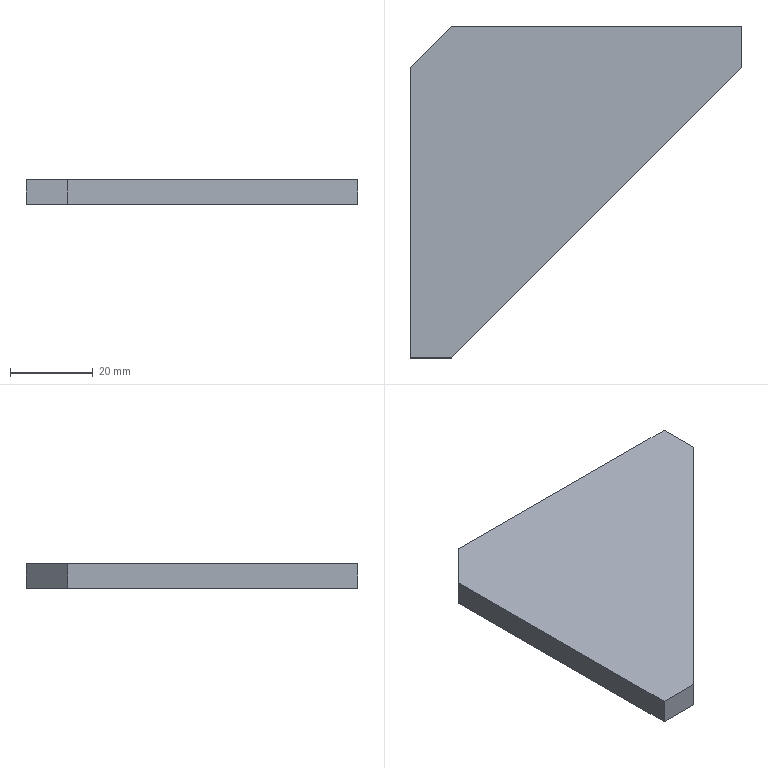Part | SolidWorks | features BaseBody 1 | 1 solid | 8 faces | box 80 x 80 x 6 mm | volume 23400 mm3 | plane 8
STEP:
#1=CARTESIAN_POINT('',(80.,-10.,0.));
#2=VERTEX_POINT('',#1);
#3=CARTESIAN_POINT('',(80.,0.,0.));
#4=VERTEX_POINT('',#3);
#5=CARTESIAN_POINT('',(80.,0.,0.));
#6=DIRECTION('',(0.,1.,0.));
#7=VECTOR('',#6,1000.);
#8=LINE('',#5,#7);
#9=EDGE_CURVE('',#2,#4,#8,.T.);
#10=ORIENTED_EDGE('',*,*,#9,.T.);
#11=CARTESIAN_POINT('',(10.,0.,0.));
#12=VERTEX_POINT('',#11);
#13=CARTESIAN_POINT('',(10.,0.,0.));
#14=DIRECTION('',(-1.,0.,0.));
#15=VECTOR('',#14,1000.);
#16=LINE('',#13,#15);
#17=EDGE_CURVE('',#4,#12,#16,.T.);
#18=ORIENTED_EDGE('',*,*,#17,.T.);
#19=CARTESIAN_POINT('',(0.,-10.,0.));
#20=VERTEX_POINT('',#19);
#21=CARTESIAN_POINT('',(0.,-10.,0.));
#22=DIRECTION('',(-0.7071,-0.7071,0.));
#23=VECTOR('',#22,1000.);
#24=LINE('',#21,#23);
#25=EDGE_CURVE('',#12,#20,#24,.T.);
#26=ORIENTED_EDGE('',*,*,#25,.T.);
#27=CARTESIAN_POINT('',(0.,-80.,0.));
#28=VERTEX_POINT('',#27);
#29=CARTESIAN_POINT('',(0.,-80.,0.));
#30=DIRECTION('',(0.,-1.,0.));
#31=VECTOR('',#30,1000.);
#32=LINE('',#29,#31);
#33=EDGE_CURVE('',#20,#28,#32,.T.);
#34=ORIENTED_EDGE('',*,*,#33,.T.);
#35=CARTESIAN_POINT('',(10.,-80.,0.));
#36=VERTEX_POINT('',#35);
#37=CARTESIAN_POINT('',(10.,-80.,0.));
#38=DIRECTION('',(1.,0.,0.));
#39=VECTOR('',#38,1000.);
#40=LINE('',#37,#39);
#41=EDGE_CURVE('',#28,#36,#40,.T.);
#42=ORIENTED_EDGE('',*,*,#41,.T.);
#43=CARTESIAN_POINT('',(80.,-10.,0.));
#44=DIRECTION('',(0.7071,0.7071,0.));
#45=VECTOR('',#44,1000.);
#46=LINE('',#43,#45);
#47=EDGE_CURVE('',#36,#2,#46,.T.);
#48=ORIENTED_EDGE('',*,*,#47,.T.);
#49=EDGE_LOOP('',(#10,#18,#26,#34,#42,#48));
#50=FACE_OUTER_BOUND('',#49,.T.);
#51=CARTESIAN_POINT('',(0.,0.,0.));
#52=DIRECTION('',(0.,0.,-1.));
#53=DIRECTION('',(0.,-1.,0.));
#54=AXIS2_PLACEMENT_3D('',#51,#52,#53);
#55=PLANE('',#54);
#56=ADVANCED_FACE('',(#50),#55,.F.);
#57=CARTESIAN_POINT('',(80.,-10.,-6.));
#58=VERTEX_POINT('',#57);
#59=CARTESIAN_POINT('',(80.,0.,-6.));
#60=VERTEX_POINT('',#59);
#61=CARTESIAN_POINT('',(80.,0.,-6.));
#62=DIRECTION('',(0.,1.,0.));
#63=VECTOR('',#62,1000.);
#64=LINE('',#61,#63);
#65=EDGE_CURVE('',#58,#60,#64,.T.);
#66=ORIENTED_EDGE('',*,*,#65,.F.);
#67=CARTESIAN_POINT('',(10.,-80.,-6.));
#68=VERTEX_POINT('',#67);
#69=CARTESIAN_POINT('',(80.,-10.,-6.));
#70=DIRECTION('',(0.7071,0.7071,0.));
#71=VECTOR('',#70,1000.);
#72=LINE('',#69,#71);
#73=EDGE_CURVE('',#68,#58,#72,.T.);
#74=ORIENTED_EDGE('',*,*,#73,.F.);
#75=CARTESIAN_POINT('',(0.,-80.,-6.));
#76=VERTEX_POINT('',#75);
#77=CARTESIAN_POINT('',(10.,-80.,-6.));
#78=DIRECTION('',(1.,0.,0.));
#79=VECTOR('',#78,1000.);
#80=LINE('',#77,#79);
#81=EDGE_CURVE('',#76,#68,#80,.T.);
#82=ORIENTED_EDGE('',*,*,#81,.F.);
#83=CARTESIAN_POINT('',(0.,-10.,-6.));
#84=VERTEX_POINT('',#83);
#85=CARTESIAN_POINT('',(0.,-80.,-6.));
#86=DIRECTION('',(0.,-1.,0.));
#87=VECTOR('',#86,1000.);
#88=LINE('',#85,#87);
#89=EDGE_CURVE('',#84,#76,#88,.T.);
#90=ORIENTED_EDGE('',*,*,#89,.F.);
#91=CARTESIAN_POINT('',(10.,0.,-6.));
#92=VERTEX_POINT('',#91);
#93=CARTESIAN_POINT('',(0.,-10.,-6.));
#94=DIRECTION('',(-0.7071,-0.7071,0.));
#95=VECTOR('',#94,1000.);
#96=LINE('',#93,#95);
#97=EDGE_CURVE('',#92,#84,#96,.T.);
#98=ORIENTED_EDGE('',*,*,#97,.F.);
#99=CARTESIAN_POINT('',(10.,0.,-6.));
#100=DIRECTION('',(-1.,0.,0.));
#101=VECTOR('',#100,1000.);
#102=LINE('',#99,#101);
#103=EDGE_CURVE('',#60,#92,#102,.T.);
#104=ORIENTED_EDGE('',*,*,#103,.F.);
#105=EDGE_LOOP('',(#66,#74,#82,#90,#98,#104));
#106=FACE_OUTER_BOUND('',#105,.T.);
#107=CARTESIAN_POINT('',(0.,0.,-6.));
#108=DIRECTION('',(0.,0.,-1.));
#109=DIRECTION('',(0.,-1.,0.));
#110=AXIS2_PLACEMENT_3D('',#107,#108,#109);
#111=PLANE('',#110);
#112=ADVANCED_FACE('',(#106),#111,.T.);
#113=ORIENTED_EDGE('',*,*,#17,.F.);
#114=CARTESIAN_POINT('',(80.,0.,-6.));
#115=DIRECTION('',(0.,0.,1.));
#116=VECTOR('',#115,1000.);
#117=LINE('',#114,#116);
#118=EDGE_CURVE('',#60,#4,#117,.T.);
#119=ORIENTED_EDGE('',*,*,#118,.F.);
#120=ORIENTED_EDGE('',*,*,#103,.T.);
#121=CARTESIAN_POINT('',(10.,0.,-6.));
#122=DIRECTION('',(0.,0.,1.));
#123=VECTOR('',#122,1000.);
#124=LINE('',#121,#123);
#125=EDGE_CURVE('',#92,#12,#124,.T.);
#126=ORIENTED_EDGE('',*,*,#125,.T.);
#127=EDGE_LOOP('',(#113,#119,#120,#126));
#128=FACE_OUTER_BOUND('',#127,.T.);
#129=CARTESIAN_POINT('',(10.,0.,-6.));
#130=DIRECTION('',(0.,1.,0.));
#131=DIRECTION('',(1.,0.,0.));
#132=AXIS2_PLACEMENT_3D('',#129,#130,#131);
#133=PLANE('',#132);
#134=ADVANCED_FACE('',(#128),#133,.T.);
#135=ORIENTED_EDGE('',*,*,#25,.F.);
#136=ORIENTED_EDGE('',*,*,#125,.F.);
#137=ORIENTED_EDGE('',*,*,#97,.T.);
#138=CARTESIAN_POINT('',(0.,-10.,-6.));
#139=DIRECTION('',(0.,0.,1.));
#140=VECTOR('',#139,1000.);
#141=LINE('',#138,#140);
#142=EDGE_CURVE('',#84,#20,#141,.T.);
#143=ORIENTED_EDGE('',*,*,#142,.T.);
#144=EDGE_LOOP('',(#135,#136,#137,#143));
#145=FACE_OUTER_BOUND('',#144,.T.);
#146=CARTESIAN_POINT('',(0.,-10.,-6.));
#147=DIRECTION('',(-0.7071,0.7071,0.));
#148=DIRECTION('',(0.,0.,1.));
#149=AXIS2_PLACEMENT_3D('',#146,#147,#148);
#150=PLANE('',#149);
#151=ADVANCED_FACE('',(#145),#150,.T.);
#152=ORIENTED_EDGE('',*,*,#33,.F.);
#153=ORIENTED_EDGE('',*,*,#142,.F.);
#154=ORIENTED_EDGE('',*,*,#89,.T.);
#155=CARTESIAN_POINT('',(0.,-80.,-6.));
#156=DIRECTION('',(0.,0.,1.));
#157=VECTOR('',#156,1000.);
#158=LINE('',#155,#157);
#159=EDGE_CURVE('',#76,#28,#158,.T.);
#160=ORIENTED_EDGE('',*,*,#159,.T.);
#161=EDGE_LOOP('',(#152,#153,#154,#160));
#162=FACE_OUTER_BOUND('',#161,.T.);
#163=CARTESIAN_POINT('',(0.,-80.,-6.));
#164=DIRECTION('',(-1.,0.,0.));
#165=DIRECTION('',(0.,0.,1.));
#166=AXIS2_PLACEMENT_3D('',#163,#164,#165);
#167=PLANE('',#166);
#168=ADVANCED_FACE('',(#162),#167,.T.);
#169=ORIENTED_EDGE('',*,*,#41,.F.);
#170=ORIENTED_EDGE('',*,*,#159,.F.);
#171=ORIENTED_EDGE('',*,*,#81,.T.);
#172=CARTESIAN_POINT('',(10.,-80.,-6.));
#173=DIRECTION('',(0.,0.,1.));
#174=VECTOR('',#173,1000.);
#175=LINE('',#172,#174);
#176=EDGE_CURVE('',#68,#36,#175,.T.);
#177=ORIENTED_EDGE('',*,*,#176,.T.);
#178=EDGE_LOOP('',(#169,#170,#171,#177));
#179=FACE_OUTER_BOUND('',#178,.T.);
#180=CARTESIAN_POINT('',(10.,-80.,-6.));
#181=DIRECTION('',(0.,-1.,0.));
#182=DIRECTION('',(0.,0.,-1.));
#183=AXIS2_PLACEMENT_3D('',#180,#181,#182);
#184=PLANE('',#183);
#185=ADVANCED_FACE('',(#179),#184,.T.);
#186=ORIENTED_EDGE('',*,*,#47,.F.);
#187=ORIENTED_EDGE('',*,*,#176,.F.);
#188=ORIENTED_EDGE('',*,*,#73,.T.);
#189=CARTESIAN_POINT('',(80.,-10.,-6.));
#190=DIRECTION('',(0.,0.,1.));
#191=VECTOR('',#190,1000.);
#192=LINE('',#189,#191);
#193=EDGE_CURVE('',#58,#2,#192,.T.);
#194=ORIENTED_EDGE('',*,*,#193,.T.);
#195=EDGE_LOOP('',(#186,#187,#188,#194));
#196=FACE_OUTER_BOUND('',#195,.T.);
#197=CARTESIAN_POINT('',(80.,-10.,-6.));
#198=DIRECTION('',(0.7071,-0.7071,0.));
#199=DIRECTION('',(0.,0.,-1.));
#200=AXIS2_PLACEMENT_3D('',#197,#198,#199);
#201=PLANE('',#200);
#202=ADVANCED_FACE('',(#196),#201,.T.);
#203=ORIENTED_EDGE('',*,*,#9,.F.);
#204=ORIENTED_EDGE('',*,*,#193,.F.);
#205=ORIENTED_EDGE('',*,*,#65,.T.);
#206=ORIENTED_EDGE('',*,*,#118,.T.);
#207=EDGE_LOOP('',(#203,#204,#205,#206));
#208=FACE_OUTER_BOUND('',#207,.T.);
#209=CARTESIAN_POINT('',(80.,0.,-6.));
#210=DIRECTION('',(1.,0.,0.));
#211=DIRECTION('',(0.,1.,0.));
#212=AXIS2_PLACEMENT_3D('',#209,#210,#211);
#213=PLANE('',#212);
#214=ADVANCED_FACE('',(#208),#213,.T.);
#215=CLOSED_SHELL('',(#56,#112,#134,#151,#168,#185,#202,#214));
#216=MANIFOLD_SOLID_BREP('',#215);
#217=CARTESIAN_POINT('',(0.,0.,0.));
#218=DIRECTION('',(0.,0.,1.));
#219=DIRECTION('',(1.,0.,0.));
#220=AXIS2_PLACEMENT_3D('',#217,#218,#219);
#221=(LENGTH_UNIT()NAMED_UNIT(*)SI_UNIT(.MILLI.,.METRE.));
#222=UNCERTAINTY_MEASURE_WITH_UNIT(LENGTH_MEASURE(0.00001),#221,'','');
#223=(NAMED_UNIT(*)PLANE_ANGLE_UNIT()SI_UNIT($,.RADIAN.));
#224=(NAMED_UNIT(*)SI_UNIT($,.STERADIAN.)SOLID_ANGLE_UNIT());
#225=(GEOMETRIC_REPRESENTATION_CONTEXT(3)GLOBAL_UNCERTAINTY_ASSIGNED_CONTEXT((#222))GLOBAL_UNIT_ASSIGNED_CONTEXT((#221,#223,#224))REPRESENTATION_CONTEXT('',''));
#226=ADVANCED_BREP_SHAPE_REPRESENTATION('',(#216,#220),#225);